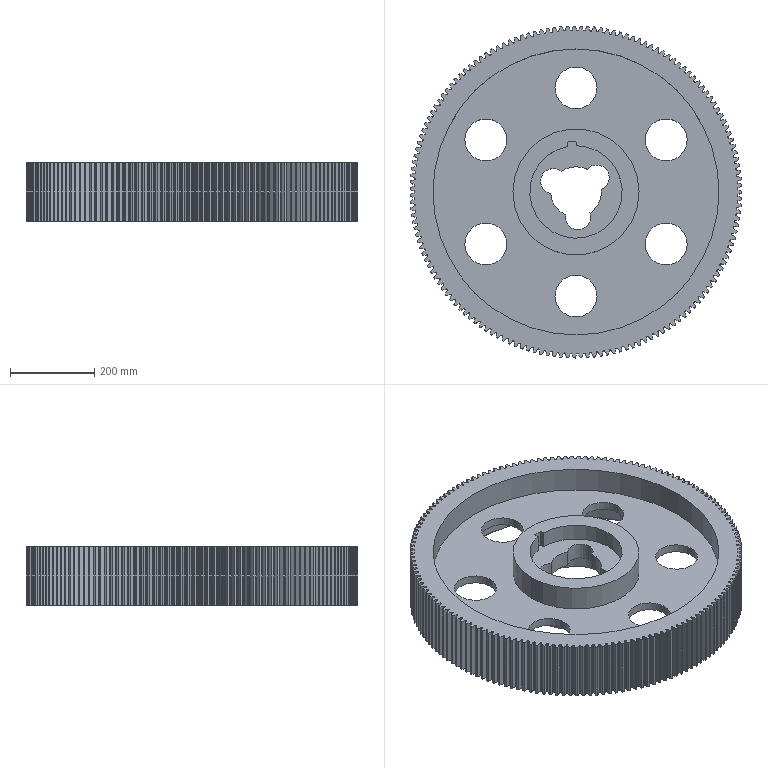Part | SolidWorks | features BaseBody 1 | 1 solid | 1208 faces | box 789.18 x 789.212 x 140 mm | volume 25623367 mm3 | cylinder 880 | plane 324 | cone 4 | commonest cylinder face diameters 3.8 x372 262.053 x157 262.284 x157 789.22 x156 100 x12 60 x7